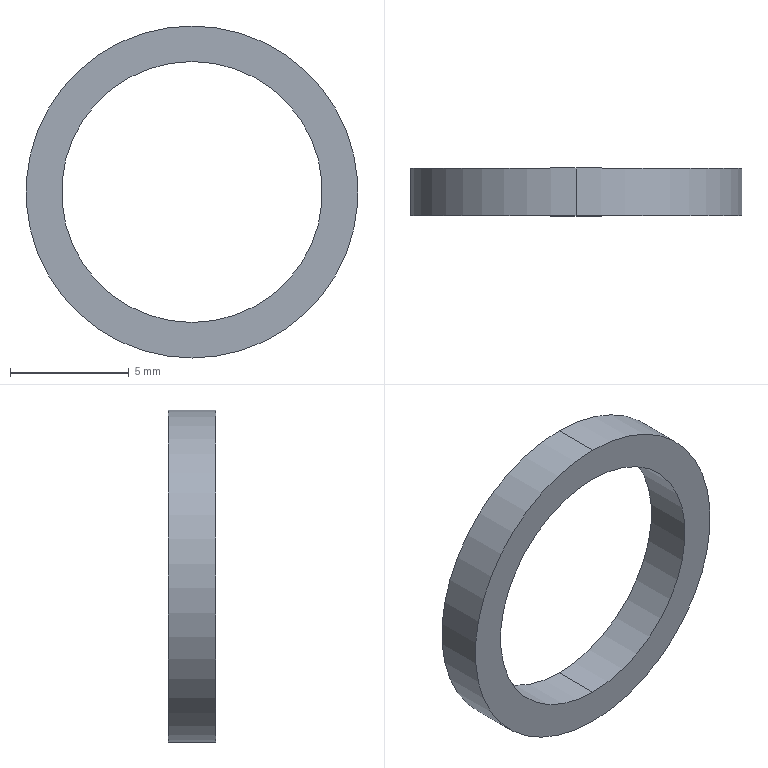Part | SolidWorks | features Extrusion 1 | 1 solid | 6 faces | box 14 x 2 x 14 mm | volume 117.81 mm3 | cylinder 4 | plane 2 | commonest cylinder face diameters 11 x2 14 x2
STEP:
#1=CARTESIAN_POINT('',(0.,1.,-5.5));
#2=VERTEX_POINT('',#1);
#3=CARTESIAN_POINT('',(0.,1.,5.5));
#4=VERTEX_POINT('',#3);
#5=CARTESIAN_POINT('',(0.,1.,0.));
#6=DIRECTION('',(0.,1.,0.));
#7=DIRECTION('',(0.,0.,1.));
#8=AXIS2_PLACEMENT_3D('',#5,#6,#7);
#9=CIRCLE('',#8,5.5);
#10=EDGE_CURVE('',#2,#4,#9,.T.);
#11=ORIENTED_EDGE('',*,*,#10,.T.);
#12=CARTESIAN_POINT('',(0.,-1.,5.5));
#13=VERTEX_POINT('',#12);
#14=CARTESIAN_POINT('',(0.,1.,5.5));
#15=DIRECTION('',(0.,-1.,0.));
#16=VECTOR('',#15,1000.);
#17=LINE('',#14,#16);
#18=EDGE_CURVE('',#4,#13,#17,.T.);
#19=ORIENTED_EDGE('',*,*,#18,.T.);
#20=CARTESIAN_POINT('',(0.,-1.,-5.5));
#21=VERTEX_POINT('',#20);
#22=CARTESIAN_POINT('',(0.,-1.,0.));
#23=DIRECTION('',(0.,1.,0.));
#24=DIRECTION('',(0.,0.,1.));
#25=AXIS2_PLACEMENT_3D('',#22,#23,#24);
#26=CIRCLE('',#25,5.5);
#27=EDGE_CURVE('',#21,#13,#26,.T.);
#28=ORIENTED_EDGE('',*,*,#27,.F.);
#29=CARTESIAN_POINT('',(0.,1.,-5.5));
#30=DIRECTION('',(0.,-1.,0.));
#31=VECTOR('',#30,1000.);
#32=LINE('',#29,#31);
#33=EDGE_CURVE('',#2,#21,#32,.T.);
#34=ORIENTED_EDGE('',*,*,#33,.F.);
#35=EDGE_LOOP('',(#11,#19,#28,#34));
#36=FACE_OUTER_BOUND('',#35,.T.);
#37=CARTESIAN_POINT('',(0.,1.,0.));
#38=DIRECTION('',(0.,-1.,0.));
#39=DIRECTION('',(0.,0.,-1.));
#40=AXIS2_PLACEMENT_3D('',#37,#38,#39);
#41=CYLINDRICAL_SURFACE('',#40,5.5);
#42=ADVANCED_FACE('',(#36),#41,.F.);
#43=CARTESIAN_POINT('',(0.,1.,7.));
#44=VERTEX_POINT('',#43);
#45=CARTESIAN_POINT('',(0.,1.,-7.));
#46=VERTEX_POINT('',#45);
#47=CARTESIAN_POINT('',(0.,1.,0.));
#48=DIRECTION('',(0.,1.,0.));
#49=DIRECTION('',(0.,0.,1.));
#50=AXIS2_PLACEMENT_3D('',#47,#48,#49);
#51=CIRCLE('',#50,7.);
#52=EDGE_CURVE('',#44,#46,#51,.T.);
#53=ORIENTED_EDGE('',*,*,#52,.F.);
#54=CARTESIAN_POINT('',(0.,-1.,7.));
#55=VERTEX_POINT('',#54);
#56=CARTESIAN_POINT('',(0.,1.,7.));
#57=DIRECTION('',(0.,-1.,0.));
#58=VECTOR('',#57,1000.);
#59=LINE('',#56,#58);
#60=EDGE_CURVE('',#44,#55,#59,.T.);
#61=ORIENTED_EDGE('',*,*,#60,.T.);
#62=CARTESIAN_POINT('',(0.,-1.,-7.));
#63=VERTEX_POINT('',#62);
#64=CARTESIAN_POINT('',(0.,-1.,0.));
#65=DIRECTION('',(0.,1.,0.));
#66=DIRECTION('',(0.,0.,1.));
#67=AXIS2_PLACEMENT_3D('',#64,#65,#66);
#68=CIRCLE('',#67,7.);
#69=EDGE_CURVE('',#55,#63,#68,.T.);
#70=ORIENTED_EDGE('',*,*,#69,.T.);
#71=CARTESIAN_POINT('',(0.,1.,-7.));
#72=DIRECTION('',(0.,-1.,0.));
#73=VECTOR('',#72,1000.);
#74=LINE('',#71,#73);
#75=EDGE_CURVE('',#46,#63,#74,.T.);
#76=ORIENTED_EDGE('',*,*,#75,.F.);
#77=EDGE_LOOP('',(#53,#61,#70,#76));
#78=FACE_OUTER_BOUND('',#77,.T.);
#79=CARTESIAN_POINT('',(0.,1.,0.));
#80=DIRECTION('',(0.,-1.,0.));
#81=DIRECTION('',(0.,0.,-1.));
#82=AXIS2_PLACEMENT_3D('',#79,#80,#81);
#83=CYLINDRICAL_SURFACE('',#82,7.);
#84=ADVANCED_FACE('',(#78),#83,.T.);
#85=CARTESIAN_POINT('',(0.,1.,0.));
#86=DIRECTION('',(0.,1.,0.));
#87=DIRECTION('',(0.,0.,1.));
#88=AXIS2_PLACEMENT_3D('',#85,#86,#87);
#89=CIRCLE('',#88,7.);
#90=EDGE_CURVE('',#46,#44,#89,.T.);
#91=ORIENTED_EDGE('',*,*,#90,.T.);
#92=ORIENTED_EDGE('',*,*,#52,.T.);
#93=EDGE_LOOP('',(#91,#92));
#94=FACE_OUTER_BOUND('',#93,.T.);
#95=ORIENTED_EDGE('',*,*,#10,.F.);
#96=CARTESIAN_POINT('',(0.,1.,0.));
#97=DIRECTION('',(0.,1.,0.));
#98=DIRECTION('',(0.,0.,1.));
#99=AXIS2_PLACEMENT_3D('',#96,#97,#98);
#100=CIRCLE('',#99,5.5);
#101=EDGE_CURVE('',#4,#2,#100,.T.);
#102=ORIENTED_EDGE('',*,*,#101,.F.);
#103=EDGE_LOOP('',(#95,#102));
#104=FACE_BOUND('',#103,.T.);
#105=CARTESIAN_POINT('',(0.,1.,0.));
#106=DIRECTION('',(0.,1.,0.));
#107=DIRECTION('',(0.,0.,1.));
#108=AXIS2_PLACEMENT_3D('',#105,#106,#107);
#109=PLANE('',#108);
#110=ADVANCED_FACE('',(#94,#104),#109,.T.);
#111=CARTESIAN_POINT('',(0.,-1.,0.));
#112=DIRECTION('',(0.,1.,0.));
#113=DIRECTION('',(0.,0.,1.));
#114=AXIS2_PLACEMENT_3D('',#111,#112,#113);
#115=CIRCLE('',#114,7.);
#116=EDGE_CURVE('',#63,#55,#115,.T.);
#117=ORIENTED_EDGE('',*,*,#116,.F.);
#118=ORIENTED_EDGE('',*,*,#69,.F.);
#119=EDGE_LOOP('',(#117,#118));
#120=FACE_OUTER_BOUND('',#119,.T.);
#121=ORIENTED_EDGE('',*,*,#27,.T.);
#122=CARTESIAN_POINT('',(0.,-1.,0.));
#123=DIRECTION('',(0.,1.,0.));
#124=DIRECTION('',(0.,0.,1.));
#125=AXIS2_PLACEMENT_3D('',#122,#123,#124);
#126=CIRCLE('',#125,5.5);
#127=EDGE_CURVE('',#13,#21,#126,.T.);
#128=ORIENTED_EDGE('',*,*,#127,.T.);
#129=EDGE_LOOP('',(#121,#128));
#130=FACE_BOUND('',#129,.T.);
#131=CARTESIAN_POINT('',(0.,-1.,0.));
#132=DIRECTION('',(0.,1.,0.));
#133=DIRECTION('',(0.,0.,1.));
#134=AXIS2_PLACEMENT_3D('',#131,#132,#133);
#135=PLANE('',#134);
#136=ADVANCED_FACE('',(#120,#130),#135,.F.);
#137=ORIENTED_EDGE('',*,*,#60,.F.);
#138=ORIENTED_EDGE('',*,*,#90,.F.);
#139=ORIENTED_EDGE('',*,*,#75,.T.);
#140=ORIENTED_EDGE('',*,*,#116,.T.);
#141=EDGE_LOOP('',(#137,#138,#139,#140));
#142=FACE_OUTER_BOUND('',#141,.T.);
#143=CARTESIAN_POINT('',(0.,1.,0.));
#144=DIRECTION('',(0.,-1.,0.));
#145=DIRECTION('',(0.,0.,-1.));
#146=AXIS2_PLACEMENT_3D('',#143,#144,#145);
#147=CYLINDRICAL_SURFACE('',#146,7.);
#148=ADVANCED_FACE('',(#142),#147,.T.);
#149=ORIENTED_EDGE('',*,*,#18,.F.);
#150=ORIENTED_EDGE('',*,*,#101,.T.);
#151=ORIENTED_EDGE('',*,*,#33,.T.);
#152=ORIENTED_EDGE('',*,*,#127,.F.);
#153=EDGE_LOOP('',(#149,#150,#151,#152));
#154=FACE_OUTER_BOUND('',#153,.T.);
#155=CARTESIAN_POINT('',(0.,1.,0.));
#156=DIRECTION('',(0.,-1.,0.));
#157=DIRECTION('',(0.,0.,-1.));
#158=AXIS2_PLACEMENT_3D('',#155,#156,#157);
#159=CYLINDRICAL_SURFACE('',#158,5.5);
#160=ADVANCED_FACE('',(#154),#159,.F.);
#161=CLOSED_SHELL('',(#42,#84,#110,#136,#148,#160));
#162=MANIFOLD_SOLID_BREP('',#161);
#163=CARTESIAN_POINT('',(0.,0.,0.));
#164=DIRECTION('',(0.,0.,1.));
#165=DIRECTION('',(1.,0.,0.));
#166=AXIS2_PLACEMENT_3D('',#163,#164,#165);
#167=(LENGTH_UNIT()NAMED_UNIT(*)SI_UNIT(.MILLI.,.METRE.));
#168=UNCERTAINTY_MEASURE_WITH_UNIT(LENGTH_MEASURE(0.00001),#167,'','');
#169=(NAMED_UNIT(*)PLANE_ANGLE_UNIT()SI_UNIT($,.RADIAN.));
#170=(NAMED_UNIT(*)SI_UNIT($,.STERADIAN.)SOLID_ANGLE_UNIT());
#171=(GEOMETRIC_REPRESENTATION_CONTEXT(3)GLOBAL_UNCERTAINTY_ASSIGNED_CONTEXT((#168))GLOBAL_UNIT_ASSIGNED_CONTEXT((#167,#169,#170))REPRESENTATION_CONTEXT('',''));
#172=ADVANCED_BREP_SHAPE_REPRESENTATION('',(#162,#166),#171);